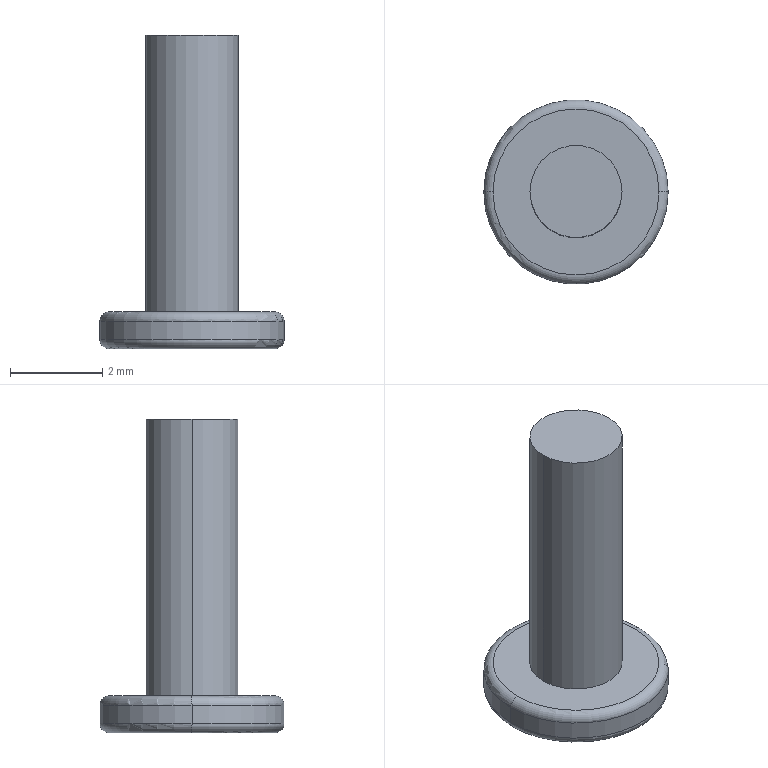Part | NX | features BREP 1 | 1 solid | 24 faces | box 4 x 4 x 6.8 mm | volume 27.69 mm3 | plane 10 | cone 6 | torus 4 | cylinder 4 | commonest cylinder face diameters 2 x2 4 x2
STEP:
#1=CARTESIAN_POINT('',(-2.,0.,0.6));
#2=VERTEX_POINT('',#1);
#3=CARTESIAN_POINT('',(2.,0.,0.6));
#4=VERTEX_POINT('',#3);
#5=CARTESIAN_POINT('',(0.,0.,0.6));
#6=DIRECTION('',(0.,0.,-1.));
#7=DIRECTION('',(1.,0.,0.));
#8=AXIS2_PLACEMENT_3D('',#5,#6,#7);
#9=CIRCLE('',#8,2.);
#10=EDGE_CURVE('',#2,#4,#9,.T.);
#11=ORIENTED_EDGE('',*,*,#10,.F.);
#12=CARTESIAN_POINT('',(-1.8,0.,0.8));
#13=VERTEX_POINT('',#12);
#14=CARTESIAN_POINT('',(-1.8,0.,0.6));
#15=DIRECTION('',(0.,1.,0.));
#16=DIRECTION('',(-1.,0.,0.));
#17=AXIS2_PLACEMENT_3D('',#14,#15,#16);
#18=CIRCLE('',#17,0.2);
#19=EDGE_CURVE('',#2,#13,#18,.T.);
#20=ORIENTED_EDGE('',*,*,#19,.T.);
#21=CARTESIAN_POINT('',(1.8,0.,0.8));
#22=VERTEX_POINT('',#21);
#23=CARTESIAN_POINT('',(0.,0.,0.8));
#24=DIRECTION('',(0.,0.,1.));
#25=DIRECTION('',(1.,0.,0.));
#26=AXIS2_PLACEMENT_3D('',#23,#24,#25);
#27=CIRCLE('',#26,1.8);
#28=EDGE_CURVE('',#22,#13,#27,.T.);
#29=ORIENTED_EDGE('',*,*,#28,.F.);
#30=CARTESIAN_POINT('',(1.8,0.,0.6));
#31=DIRECTION('',(0.,-1.,0.));
#32=DIRECTION('',(0.,0.,-1.));
#33=AXIS2_PLACEMENT_3D('',#30,#31,#32);
#34=CIRCLE('',#33,0.2);
#35=EDGE_CURVE('',#4,#22,#34,.T.);
#36=ORIENTED_EDGE('',*,*,#35,.F.);
#37=EDGE_LOOP('',(#11,#20,#29,#36));
#38=FACE_BOUND('',#37,.T.);
#39=CARTESIAN_POINT('',(0.,0.,0.6));
#40=DIRECTION('',(0.,0.,1.));
#41=DIRECTION('',(-1.,0.,0.));
#42=AXIS2_PLACEMENT_3D('',#39,#40,#41);
#43=TOROIDAL_SURFACE('',#42,1.8,0.2);
#44=ADVANCED_FACE('',(#38),#43,.T.);
#45=CARTESIAN_POINT('',(-1.8,0.,0.));
#46=VERTEX_POINT('',#45);
#47=CARTESIAN_POINT('',(1.8,0.,0.));
#48=VERTEX_POINT('',#47);
#49=CARTESIAN_POINT('',(0.,0.,0.));
#50=DIRECTION('',(0.,0.,-1.));
#51=DIRECTION('',(1.,0.,0.));
#52=AXIS2_PLACEMENT_3D('',#49,#50,#51);
#53=CIRCLE('',#52,1.8);
#54=EDGE_CURVE('',#46,#48,#53,.T.);
#55=ORIENTED_EDGE('',*,*,#54,.F.);
#56=CARTESIAN_POINT('',(-2.,0.,0.2));
#57=VERTEX_POINT('',#56);
#58=CARTESIAN_POINT('',(-1.8,0.,0.2));
#59=DIRECTION('',(0.,1.,0.));
#60=DIRECTION('',(-1.,0.,0.));
#61=AXIS2_PLACEMENT_3D('',#58,#59,#60);
#62=CIRCLE('',#61,0.2);
#63=EDGE_CURVE('',#46,#57,#62,.T.);
#64=ORIENTED_EDGE('',*,*,#63,.T.);
#65=CARTESIAN_POINT('',(2.,0.,0.2));
#66=VERTEX_POINT('',#65);
#67=CARTESIAN_POINT('',(0.,0.,0.2));
#68=DIRECTION('',(0.,0.,1.));
#69=DIRECTION('',(1.,0.,0.));
#70=AXIS2_PLACEMENT_3D('',#67,#68,#69);
#71=CIRCLE('',#70,2.);
#72=EDGE_CURVE('',#66,#57,#71,.T.);
#73=ORIENTED_EDGE('',*,*,#72,.F.);
#74=CARTESIAN_POINT('',(1.8,0.,0.2));
#75=DIRECTION('',(0.,-1.,0.));
#76=DIRECTION('',(0.,0.,-1.));
#77=AXIS2_PLACEMENT_3D('',#74,#75,#76);
#78=CIRCLE('',#77,0.2);
#79=EDGE_CURVE('',#48,#66,#78,.T.);
#80=ORIENTED_EDGE('',*,*,#79,.F.);
#81=EDGE_LOOP('',(#55,#64,#73,#80));
#82=FACE_BOUND('',#81,.T.);
#83=CARTESIAN_POINT('',(0.,0.,0.2));
#84=DIRECTION('',(0.,0.,1.));
#85=DIRECTION('',(-1.,0.,0.));
#86=AXIS2_PLACEMENT_3D('',#83,#84,#85);
#87=TOROIDAL_SURFACE('',#86,1.8,0.2);
#88=ADVANCED_FACE('',(#82),#87,.T.);
#89=CARTESIAN_POINT('',(1.,0.,6.8));
#90=VERTEX_POINT('',#89);
#91=CARTESIAN_POINT('',(-1.,0.,6.8));
#92=VERTEX_POINT('',#91);
#93=CARTESIAN_POINT('',(0.,0.,6.8));
#94=DIRECTION('',(0.,0.,1.));
#95=DIRECTION('',(1.,0.,0.));
#96=AXIS2_PLACEMENT_3D('',#93,#94,#95);
#97=CIRCLE('',#96,1.);
#98=EDGE_CURVE('',#90,#92,#97,.T.);
#99=ORIENTED_EDGE('',*,*,#98,.F.);
#100=CARTESIAN_POINT('',(1.,0.,0.8));
#101=VERTEX_POINT('',#100);
#102=CARTESIAN_POINT('',(1.,0.,6.8));
#103=DIRECTION('',(0.,0.,-1.));
#104=VECTOR('',#103,1000.);
#105=LINE('',#102,#104);
#106=EDGE_CURVE('',#101,#90,#105,.F.);
#107=ORIENTED_EDGE('',*,*,#106,.F.);
#108=CARTESIAN_POINT('',(-1.,0.,0.8));
#109=VERTEX_POINT('',#108);
#110=CARTESIAN_POINT('',(0.,0.,0.8));
#111=DIRECTION('',(0.,0.,1.));
#112=DIRECTION('',(1.,0.,0.));
#113=AXIS2_PLACEMENT_3D('',#110,#111,#112);
#114=CIRCLE('',#113,1.);
#115=EDGE_CURVE('',#101,#109,#114,.T.);
#116=ORIENTED_EDGE('',*,*,#115,.T.);
#117=CARTESIAN_POINT('',(-1.,0.,6.8));
#118=DIRECTION('',(0.,0.,-1.));
#119=VECTOR('',#118,1000.);
#120=LINE('',#117,#119);
#121=EDGE_CURVE('',#109,#92,#120,.F.);
#122=ORIENTED_EDGE('',*,*,#121,.T.);
#123=EDGE_LOOP('',(#99,#107,#116,#122));
#124=FACE_BOUND('',#123,.T.);
#125=CARTESIAN_POINT('',(0.,0.,6.8));
#126=DIRECTION('',(0.,0.,-1.));
#127=DIRECTION('',(1.,0.,0.));
#128=AXIS2_PLACEMENT_3D('',#125,#126,#127);
#129=CYLINDRICAL_SURFACE('',#128,1.);
#130=ADVANCED_FACE('',(#124),#129,.T.);
#131=ORIENTED_EDGE('',*,*,#10,.T.);
#132=CARTESIAN_POINT('',(2.,0.,0.8));
#133=DIRECTION('',(0.,0.,-1.));
#134=VECTOR('',#133,1000.);
#135=LINE('',#132,#134);
#136=EDGE_CURVE('',#66,#4,#135,.F.);
#137=ORIENTED_EDGE('',*,*,#136,.F.);
#138=ORIENTED_EDGE('',*,*,#72,.T.);
#139=CARTESIAN_POINT('',(-2.,0.,0.8));
#140=DIRECTION('',(0.,0.,-1.));
#141=VECTOR('',#140,1000.);
#142=LINE('',#139,#141);
#143=EDGE_CURVE('',#57,#2,#142,.F.);
#144=ORIENTED_EDGE('',*,*,#143,.T.);
#145=EDGE_LOOP('',(#131,#137,#138,#144));
#146=FACE_BOUND('',#145,.T.);
#147=CARTESIAN_POINT('',(0.,0.,0.8));
#148=DIRECTION('',(0.,0.,-1.));
#149=DIRECTION('',(1.,0.,0.));
#150=AXIS2_PLACEMENT_3D('',#147,#148,#149);
#151=CYLINDRICAL_SURFACE('',#150,2.);
#152=ADVANCED_FACE('',(#146),#151,.T.);
#153=ORIENTED_EDGE('',*,*,#136,.T.);
#154=CARTESIAN_POINT('',(0.,0.,0.6));
#155=DIRECTION('',(0.,0.,-1.));
#156=DIRECTION('',(1.,0.,0.));
#157=AXIS2_PLACEMENT_3D('',#154,#155,#156);
#158=CIRCLE('',#157,2.);
#159=EDGE_CURVE('',#4,#2,#158,.T.);
#160=ORIENTED_EDGE('',*,*,#159,.T.);
#161=ORIENTED_EDGE('',*,*,#143,.F.);
#162=CARTESIAN_POINT('',(0.,0.,0.2));
#163=DIRECTION('',(0.,0.,1.));
#164=DIRECTION('',(1.,0.,0.));
#165=AXIS2_PLACEMENT_3D('',#162,#163,#164);
#166=CIRCLE('',#165,2.);
#167=EDGE_CURVE('',#57,#66,#166,.T.);
#168=ORIENTED_EDGE('',*,*,#167,.T.);
#169=EDGE_LOOP('',(#153,#160,#161,#168));
#170=FACE_BOUND('',#169,.T.);
#171=CARTESIAN_POINT('',(0.,0.,0.8));
#172=DIRECTION('',(0.,0.,-1.));
#173=DIRECTION('',(1.,0.,0.));
#174=AXIS2_PLACEMENT_3D('',#171,#172,#173);
#175=CYLINDRICAL_SURFACE('',#174,2.);
#176=ADVANCED_FACE('',(#170),#175,.T.);
#177=ORIENTED_EDGE('',*,*,#28,.T.);
#178=CARTESIAN_POINT('',(0.,0.,0.8));
#179=DIRECTION('',(0.,0.,1.));
#180=DIRECTION('',(1.,0.,0.));
#181=AXIS2_PLACEMENT_3D('',#178,#179,#180);
#182=CIRCLE('',#181,1.8);
#183=EDGE_CURVE('',#13,#22,#182,.T.);
#184=ORIENTED_EDGE('',*,*,#183,.T.);
#185=EDGE_LOOP('',(#177,#184));
#186=FACE_BOUND('',#185,.T.);
#187=CARTESIAN_POINT('',(0.,0.,0.8));
#188=DIRECTION('',(0.,0.,1.));
#189=DIRECTION('',(1.,0.,0.));
#190=AXIS2_PLACEMENT_3D('',#187,#188,#189);
#191=CIRCLE('',#190,1.);
#192=EDGE_CURVE('',#109,#101,#191,.T.);
#193=ORIENTED_EDGE('',*,*,#192,.F.);
#194=ORIENTED_EDGE('',*,*,#115,.F.);
#195=EDGE_LOOP('',(#193,#194));
#196=FACE_BOUND('',#195,.T.);
#197=CARTESIAN_POINT('',(0.,0.,0.8));
#198=DIRECTION('',(0.,0.,1.));
#199=DIRECTION('',(-1.,0.,0.));
#200=AXIS2_PLACEMENT_3D('',#197,#198,#199);
#201=PLANE('',#200);
#202=ADVANCED_FACE('',(#186,#196),#201,.T.);
#203=CARTESIAN_POINT('',(0.,0.,0.));
#204=DIRECTION('',(0.,0.,-1.));
#205=DIRECTION('',(1.,0.,0.));
#206=AXIS2_PLACEMENT_3D('',#203,#204,#205);
#207=CIRCLE('',#206,1.8);
#208=EDGE_CURVE('',#48,#46,#207,.T.);
#209=ORIENTED_EDGE('',*,*,#208,.T.);
#210=ORIENTED_EDGE('',*,*,#54,.T.);
#211=EDGE_LOOP('',(#209,#210));
#212=FACE_BOUND('',#211,.T.);
#213=CARTESIAN_POINT('',(0.866,0.,0.));
#214=VERTEX_POINT('',#213);
#215=CARTESIAN_POINT('',(0.433,-0.75,0.));
#216=VERTEX_POINT('',#215);
#217=CARTESIAN_POINT('',(0.,0.,0.));
#218=DIRECTION('',(0.,0.,-1.));
#219=DIRECTION('',(-1.,0.,0.));
#220=AXIS2_PLACEMENT_3D('',#217,#218,#219);
#221=CIRCLE('',#220,0.866);
#222=EDGE_CURVE('',#214,#216,#221,.T.);
#223=ORIENTED_EDGE('',*,*,#222,.F.);
#224=CARTESIAN_POINT('',(0.433,0.75,0.));
#225=VERTEX_POINT('',#224);
#226=CARTESIAN_POINT('',(0.,0.,0.));
#227=DIRECTION('',(0.,0.,-1.));
#228=DIRECTION('',(-1.,0.,0.));
#229=AXIS2_PLACEMENT_3D('',#226,#227,#228);
#230=CIRCLE('',#229,0.866);
#231=EDGE_CURVE('',#225,#214,#230,.T.);
#232=ORIENTED_EDGE('',*,*,#231,.F.);
#233=CARTESIAN_POINT('',(-0.433,0.75,0.));
#234=VERTEX_POINT('',#233);
#235=CARTESIAN_POINT('',(0.,0.,0.));
#236=DIRECTION('',(0.,0.,-1.));
#237=DIRECTION('',(-1.,0.,0.));
#238=AXIS2_PLACEMENT_3D('',#235,#236,#237);
#239=CIRCLE('',#238,0.866);
#240=EDGE_CURVE('',#234,#225,#239,.T.);
#241=ORIENTED_EDGE('',*,*,#240,.F.);
#242=CARTESIAN_POINT('',(-0.866,0.,0.));
#243=VERTEX_POINT('',#242);
#244=CARTESIAN_POINT('',(0.,0.,0.));
#245=DIRECTION('',(0.,0.,-1.));
#246=DIRECTION('',(-1.,0.,0.));
#247=AXIS2_PLACEMENT_3D('',#244,#245,#246);
#248=CIRCLE('',#247,0.866);
#249=EDGE_CURVE('',#243,#234,#248,.T.);
#250=ORIENTED_EDGE('',*,*,#249,.F.);
#251=CARTESIAN_POINT('',(-0.433,-0.75,0.));
#252=VERTEX_POINT('',#251);
#253=CARTESIAN_POINT('',(0.,0.,0.));
#254=DIRECTION('',(0.,0.,-1.));
#255=DIRECTION('',(-1.,0.,0.));
#256=AXIS2_PLACEMENT_3D('',#253,#254,#255);
#257=CIRCLE('',#256,0.866);
#258=EDGE_CURVE('',#252,#243,#257,.T.);
#259=ORIENTED_EDGE('',*,*,#258,.F.);
#260=CARTESIAN_POINT('',(0.,0.,0.));
#261=DIRECTION('',(0.,0.,-1.));
#262=DIRECTION('',(-1.,0.,0.));
#263=AXIS2_PLACEMENT_3D('',#260,#261,#262);
#264=CIRCLE('',#263,0.866);
#265=EDGE_CURVE('',#216,#252,#264,.T.);
#266=ORIENTED_EDGE('',*,*,#265,.F.);
#267=EDGE_LOOP('',(#223,#232,#241,#250,#259,#266));
#268=FACE_BOUND('',#267,.T.);
#269=CARTESIAN_POINT('',(0.,0.,0.));
#270=DIRECTION('',(0.,0.,1.));
#271=DIRECTION('',(-1.,0.,0.));
#272=AXIS2_PLACEMENT_3D('',#269,#270,#271);
#273=PLANE('',#272);
#274=ADVANCED_FACE('',(#212,#268),#273,.F.);
#275=ORIENTED_EDGE('',*,*,#106,.T.);
#276=CARTESIAN_POINT('',(0.,0.,6.8));
#277=DIRECTION('',(0.,0.,1.));
#278=DIRECTION('',(1.,0.,0.));
#279=AXIS2_PLACEMENT_3D('',#276,#277,#278);
#280=CIRCLE('',#279,1.);
#281=EDGE_CURVE('',#92,#90,#280,.T.);
#282=ORIENTED_EDGE('',*,*,#281,.F.);
#283=ORIENTED_EDGE('',*,*,#121,.F.);
#284=ORIENTED_EDGE('',*,*,#192,.T.);
#285=EDGE_LOOP('',(#275,#282,#283,#284));
#286=FACE_BOUND('',#285,.T.);
#287=CARTESIAN_POINT('',(0.,0.,6.8));
#288=DIRECTION('',(0.,0.,-1.));
#289=DIRECTION('',(1.,0.,0.));
#290=AXIS2_PLACEMENT_3D('',#287,#288,#289);
#291=CYLINDRICAL_SURFACE('',#290,1.);
#292=ADVANCED_FACE('',(#286),#291,.T.);
#293=ORIENTED_EDGE('',*,*,#281,.T.);
#294=ORIENTED_EDGE('',*,*,#98,.T.);
#295=EDGE_LOOP('',(#293,#294));
#296=FACE_BOUND('',#295,.T.);
#297=CARTESIAN_POINT('',(0.,0.,6.8));
#298=DIRECTION('',(0.,0.,1.));
#299=DIRECTION('',(-1.,0.,0.));
#300=AXIS2_PLACEMENT_3D('',#297,#298,#299);
#301=PLANE('',#300);
#302=ADVANCED_FACE('',(#296),#301,.T.);
#303=ORIENTED_EDGE('',*,*,#249,.T.);
#304=CARTESIAN_POINT('',(-0.866,0.,0.));
#305=CARTESIAN_POINT('',(-0.7307,0.2344,0.1353));
#306=CARTESIAN_POINT('',(-0.5691,0.5142,0.1361));
#307=CARTESIAN_POINT('',(-0.433,0.75,0.));
#308=B_SPLINE_CURVE_WITH_KNOTS('',3,(#304,#305,#306,#307),.UNSPECIFIED.,.F.,.F.,(4,4),(0.,0.0008946),.UNSPECIFIED.);
#309=EDGE_CURVE('',#243,#234,#308,.T.);
#310=ORIENTED_EDGE('',*,*,#309,.F.);
#311=EDGE_LOOP('',(#303,#310));
#312=FACE_BOUND('',#311,.T.);
#313=CARTESIAN_POINT('',(0.,0.,0.));
#314=DIRECTION('',(0.,0.,-1.));
#315=DIRECTION('',(1.,0.,0.));
#316=AXIS2_PLACEMENT_3D('',#313,#314,#315);
#317=CONICAL_SURFACE('',#316,0.866,0.7854);
#318=ADVANCED_FACE('',(#312),#317,.F.);
#319=ORIENTED_EDGE('',*,*,#240,.T.);
#320=CARTESIAN_POINT('',(-0.433,0.75,0.));
#321=CARTESIAN_POINT('',(-0.1624,0.75,0.1353));
#322=CARTESIAN_POINT('',(0.1608,0.75,0.1361));
#323=CARTESIAN_POINT('',(0.433,0.75,0.));
#324=B_SPLINE_CURVE_WITH_KNOTS('',3,(#320,#321,#322,#323),.UNSPECIFIED.,.F.,.F.,(4,4),(0.,0.0008946),.UNSPECIFIED.);
#325=EDGE_CURVE('',#234,#225,#324,.T.);
#326=ORIENTED_EDGE('',*,*,#325,.F.);
#327=EDGE_LOOP('',(#319,#326));
#328=FACE_BOUND('',#327,.T.);
#329=CARTESIAN_POINT('',(0.,0.,0.));
#330=DIRECTION('',(0.,0.,-1.));
#331=DIRECTION('',(1.,0.,0.));
#332=AXIS2_PLACEMENT_3D('',#329,#330,#331);
#333=CONICAL_SURFACE('',#332,0.866,0.7854);
#334=ADVANCED_FACE('',(#328),#333,.F.);
#335=ORIENTED_EDGE('',*,*,#231,.T.);
#336=CARTESIAN_POINT('',(0.433,0.75,0.));
#337=CARTESIAN_POINT('',(0.5683,0.5156,0.1353));
#338=CARTESIAN_POINT('',(0.7299,0.2358,0.1361));
#339=CARTESIAN_POINT('',(0.866,0.,0.));
#340=B_SPLINE_CURVE_WITH_KNOTS('',3,(#336,#337,#338,#339),.UNSPECIFIED.,.F.,.F.,(4,4),(0.,0.0008946),.UNSPECIFIED.);
#341=EDGE_CURVE('',#225,#214,#340,.T.);
#342=ORIENTED_EDGE('',*,*,#341,.F.);
#343=EDGE_LOOP('',(#335,#342));
#344=FACE_BOUND('',#343,.T.);
#345=CARTESIAN_POINT('',(0.,0.,0.));
#346=DIRECTION('',(0.,0.,-1.));
#347=DIRECTION('',(1.,0.,0.));
#348=AXIS2_PLACEMENT_3D('',#345,#346,#347);
#349=CONICAL_SURFACE('',#348,0.866,0.7854);
#350=ADVANCED_FACE('',(#344),#349,.F.);
#351=ORIENTED_EDGE('',*,*,#222,.T.);
#352=CARTESIAN_POINT('',(0.866,0.,0.));
#353=CARTESIAN_POINT('',(0.7307,-0.2344,0.1353));
#354=CARTESIAN_POINT('',(0.5691,-0.5142,0.1361));
#355=CARTESIAN_POINT('',(0.433,-0.75,0.));
#356=B_SPLINE_CURVE_WITH_KNOTS('',3,(#352,#353,#354,#355),.UNSPECIFIED.,.F.,.F.,(4,4),(0.,0.0008946),.UNSPECIFIED.);
#357=EDGE_CURVE('',#214,#216,#356,.T.);
#358=ORIENTED_EDGE('',*,*,#357,.F.);
#359=EDGE_LOOP('',(#351,#358));
#360=FACE_BOUND('',#359,.T.);
#361=CARTESIAN_POINT('',(0.,0.,0.));
#362=DIRECTION('',(0.,0.,-1.));
#363=DIRECTION('',(1.,0.,0.));
#364=AXIS2_PLACEMENT_3D('',#361,#362,#363);
#365=CONICAL_SURFACE('',#364,0.866,0.7854);
#366=ADVANCED_FACE('',(#360),#365,.F.);
#367=ORIENTED_EDGE('',*,*,#265,.T.);
#368=CARTESIAN_POINT('',(0.433,-0.75,0.));
#369=CARTESIAN_POINT('',(0.1624,-0.75,0.1353));
#370=CARTESIAN_POINT('',(-0.1608,-0.75,0.1361));
#371=CARTESIAN_POINT('',(-0.433,-0.75,0.));
#372=B_SPLINE_CURVE_WITH_KNOTS('',3,(#368,#369,#370,#371),.UNSPECIFIED.,.F.,.F.,(4,4),(0.,0.0008946),.UNSPECIFIED.);
#373=EDGE_CURVE('',#216,#252,#372,.T.);
#374=ORIENTED_EDGE('',*,*,#373,.F.);
#375=EDGE_LOOP('',(#367,#374));
#376=FACE_BOUND('',#375,.T.);
#377=CARTESIAN_POINT('',(0.,0.,0.));
#378=DIRECTION('',(0.,0.,-1.));
#379=DIRECTION('',(1.,0.,0.));
#380=AXIS2_PLACEMENT_3D('',#377,#378,#379);
#381=CONICAL_SURFACE('',#380,0.866,0.7854);
#382=ADVANCED_FACE('',(#376),#381,.F.);
#383=ORIENTED_EDGE('',*,*,#258,.T.);
#384=CARTESIAN_POINT('',(-0.433,-0.75,0.));
#385=CARTESIAN_POINT('',(-0.5683,-0.5156,0.1353));
#386=CARTESIAN_POINT('',(-0.7299,-0.2358,0.1361));
#387=CARTESIAN_POINT('',(-0.866,0.,0.));
#388=B_SPLINE_CURVE_WITH_KNOTS('',3,(#384,#385,#386,#387),.UNSPECIFIED.,.F.,.F.,(4,4),(0.,0.0008946),.UNSPECIFIED.);
#389=EDGE_CURVE('',#252,#243,#388,.T.);
#390=ORIENTED_EDGE('',*,*,#389,.F.);
#391=EDGE_LOOP('',(#383,#390));
#392=FACE_BOUND('',#391,.T.);
#393=CARTESIAN_POINT('',(0.,0.,0.));
#394=DIRECTION('',(0.,0.,-1.));
#395=DIRECTION('',(1.,0.,0.));
#396=AXIS2_PLACEMENT_3D('',#393,#394,#395);
#397=CONICAL_SURFACE('',#396,0.866,0.7854);
#398=ADVANCED_FACE('',(#392),#397,.F.);
#399=CARTESIAN_POINT('',(-0.433,-0.75,0.5));
#400=VERTEX_POINT('',#399);
#401=CARTESIAN_POINT('',(-0.866,0.,0.5));
#402=VERTEX_POINT('',#401);
#403=CARTESIAN_POINT('',(-0.433,-0.75,0.5));
#404=DIRECTION('',(-0.5,0.866,0.));
#405=VECTOR('',#404,1000.);
#406=LINE('',#403,#405);
#407=EDGE_CURVE('',#400,#402,#406,.T.);
#408=ORIENTED_EDGE('',*,*,#407,.T.);
#409=CARTESIAN_POINT('',(-0.433,0.75,0.5));
#410=VERTEX_POINT('',#409);
#411=CARTESIAN_POINT('',(-0.866,0.,0.5));
#412=DIRECTION('',(0.5,0.866,0.));
#413=VECTOR('',#412,1000.);
#414=LINE('',#411,#413);
#415=EDGE_CURVE('',#402,#410,#414,.T.);
#416=ORIENTED_EDGE('',*,*,#415,.T.);
#417=CARTESIAN_POINT('',(0.433,0.75,0.5));
#418=VERTEX_POINT('',#417);
#419=CARTESIAN_POINT('',(-0.433,0.75,0.5));
#420=DIRECTION('',(1.,0.,0.));
#421=VECTOR('',#420,1000.);
#422=LINE('',#419,#421);
#423=EDGE_CURVE('',#410,#418,#422,.T.);
#424=ORIENTED_EDGE('',*,*,#423,.T.);
#425=CARTESIAN_POINT('',(0.866,0.,0.5));
#426=VERTEX_POINT('',#425);
#427=CARTESIAN_POINT('',(0.433,0.75,0.5));
#428=DIRECTION('',(0.5,-0.866,0.));
#429=VECTOR('',#428,1000.);
#430=LINE('',#427,#429);
#431=EDGE_CURVE('',#418,#426,#430,.T.);
#432=ORIENTED_EDGE('',*,*,#431,.T.);
#433=CARTESIAN_POINT('',(0.433,-0.75,0.5));
#434=VERTEX_POINT('',#433);
#435=CARTESIAN_POINT('',(0.866,0.,0.5));
#436=DIRECTION('',(-0.5,-0.866,0.));
#437=VECTOR('',#436,1000.);
#438=LINE('',#435,#437);
#439=EDGE_CURVE('',#426,#434,#438,.T.);
#440=ORIENTED_EDGE('',*,*,#439,.T.);
#441=CARTESIAN_POINT('',(0.433,-0.75,0.5));
#442=DIRECTION('',(-1.,0.,0.));
#443=VECTOR('',#442,1000.);
#444=LINE('',#441,#443);
#445=EDGE_CURVE('',#434,#400,#444,.T.);
#446=ORIENTED_EDGE('',*,*,#445,.T.);
#447=EDGE_LOOP('',(#408,#416,#424,#432,#440,#446));
#448=FACE_BOUND('',#447,.T.);
#449=CARTESIAN_POINT('',(0.,0.,0.5));
#450=DIRECTION('',(0.,0.,-1.));
#451=DIRECTION('',(0.,1.,0.));
#452=AXIS2_PLACEMENT_3D('',#449,#450,#451);
#453=PLANE('',#452);
#454=ADVANCED_FACE('',(#448),#453,.T.);
#455=CARTESIAN_POINT('',(-0.866,0.,0.5));
#456=DIRECTION('',(0.,0.,-1.));
#457=VECTOR('',#456,1000.);
#458=LINE('',#455,#457);
#459=EDGE_CURVE('',#402,#243,#458,.T.);
#460=ORIENTED_EDGE('',*,*,#459,.T.);
#461=ORIENTED_EDGE('',*,*,#309,.T.);
#462=CARTESIAN_POINT('',(-0.433,0.75,0.5));
#463=DIRECTION('',(0.,0.,-1.));
#464=VECTOR('',#463,1000.);
#465=LINE('',#462,#464);
#466=EDGE_CURVE('',#410,#234,#465,.T.);
#467=ORIENTED_EDGE('',*,*,#466,.F.);
#468=ORIENTED_EDGE('',*,*,#415,.F.);
#469=EDGE_LOOP('',(#460,#461,#467,#468));
#470=FACE_BOUND('',#469,.T.);
#471=CARTESIAN_POINT('',(-0.866,0.,0.5));
#472=DIRECTION('',(-0.866,0.5,0.));
#473=DIRECTION('',(0.,0.,-1.));
#474=AXIS2_PLACEMENT_3D('',#471,#472,#473);
#475=PLANE('',#474);
#476=ADVANCED_FACE('',(#470),#475,.F.);
#477=ORIENTED_EDGE('',*,*,#466,.T.);
#478=ORIENTED_EDGE('',*,*,#325,.T.);
#479=CARTESIAN_POINT('',(0.433,0.75,0.5));
#480=DIRECTION('',(0.,0.,-1.));
#481=VECTOR('',#480,1000.);
#482=LINE('',#479,#481);
#483=EDGE_CURVE('',#418,#225,#482,.T.);
#484=ORIENTED_EDGE('',*,*,#483,.F.);
#485=ORIENTED_EDGE('',*,*,#423,.F.);
#486=EDGE_LOOP('',(#477,#478,#484,#485));
#487=FACE_BOUND('',#486,.T.);
#488=CARTESIAN_POINT('',(-0.433,0.75,0.5));
#489=DIRECTION('',(0.,1.,0.));
#490=DIRECTION('',(-1.,0.,0.));
#491=AXIS2_PLACEMENT_3D('',#488,#489,#490);
#492=PLANE('',#491);
#493=ADVANCED_FACE('',(#487),#492,.F.);
#494=ORIENTED_EDGE('',*,*,#483,.T.);
#495=ORIENTED_EDGE('',*,*,#341,.T.);
#496=CARTESIAN_POINT('',(0.866,0.,0.5));
#497=DIRECTION('',(0.,0.,-1.));
#498=VECTOR('',#497,1000.);
#499=LINE('',#496,#498);
#500=EDGE_CURVE('',#426,#214,#499,.T.);
#501=ORIENTED_EDGE('',*,*,#500,.F.);
#502=ORIENTED_EDGE('',*,*,#431,.F.);
#503=EDGE_LOOP('',(#494,#495,#501,#502));
#504=FACE_BOUND('',#503,.T.);
#505=CARTESIAN_POINT('',(0.433,0.75,0.5));
#506=DIRECTION('',(0.866,0.5,0.));
#507=DIRECTION('',(0.,0.,1.));
#508=AXIS2_PLACEMENT_3D('',#505,#506,#507);
#509=PLANE('',#508);
#510=ADVANCED_FACE('',(#504),#509,.F.);
#511=ORIENTED_EDGE('',*,*,#500,.T.);
#512=ORIENTED_EDGE('',*,*,#357,.T.);
#513=CARTESIAN_POINT('',(0.433,-0.75,0.5));
#514=DIRECTION('',(0.,0.,-1.));
#515=VECTOR('',#514,1000.);
#516=LINE('',#513,#515);
#517=EDGE_CURVE('',#434,#216,#516,.T.);
#518=ORIENTED_EDGE('',*,*,#517,.F.);
#519=ORIENTED_EDGE('',*,*,#439,.F.);
#520=EDGE_LOOP('',(#511,#512,#518,#519));
#521=FACE_BOUND('',#520,.T.);
#522=CARTESIAN_POINT('',(0.866,0.,0.5));
#523=DIRECTION('',(0.866,-0.5,0.));
#524=DIRECTION('',(0.,0.,1.));
#525=AXIS2_PLACEMENT_3D('',#522,#523,#524);
#526=PLANE('',#525);
#527=ADVANCED_FACE('',(#521),#526,.F.);
#528=ORIENTED_EDGE('',*,*,#517,.T.);
#529=ORIENTED_EDGE('',*,*,#373,.T.);
#530=CARTESIAN_POINT('',(-0.433,-0.75,0.5));
#531=DIRECTION('',(0.,0.,-1.));
#532=VECTOR('',#531,1000.);
#533=LINE('',#530,#532);
#534=EDGE_CURVE('',#400,#252,#533,.T.);
#535=ORIENTED_EDGE('',*,*,#534,.F.);
#536=ORIENTED_EDGE('',*,*,#445,.F.);
#537=EDGE_LOOP('',(#528,#529,#535,#536));
#538=FACE_BOUND('',#537,.T.);
#539=CARTESIAN_POINT('',(0.433,-0.75,0.5));
#540=DIRECTION('',(0.,-1.,0.));
#541=DIRECTION('',(0.,0.,1.));
#542=AXIS2_PLACEMENT_3D('',#539,#540,#541);
#543=PLANE('',#542);
#544=ADVANCED_FACE('',(#538),#543,.F.);
#545=ORIENTED_EDGE('',*,*,#534,.T.);
#546=ORIENTED_EDGE('',*,*,#389,.T.);
#547=ORIENTED_EDGE('',*,*,#459,.F.);
#548=ORIENTED_EDGE('',*,*,#407,.F.);
#549=EDGE_LOOP('',(#545,#546,#547,#548));
#550=FACE_BOUND('',#549,.T.);
#551=CARTESIAN_POINT('',(-0.433,-0.75,0.5));
#552=DIRECTION('',(-0.866,-0.5,0.));
#553=DIRECTION('',(0.5,-0.866,0.));
#554=AXIS2_PLACEMENT_3D('',#551,#552,#553);
#555=PLANE('',#554);
#556=ADVANCED_FACE('',(#550),#555,.F.);
#557=ORIENTED_EDGE('',*,*,#63,.F.);
#558=ORIENTED_EDGE('',*,*,#208,.F.);
#559=ORIENTED_EDGE('',*,*,#79,.T.);
#560=ORIENTED_EDGE('',*,*,#167,.F.);
#561=EDGE_LOOP('',(#557,#558,#559,#560));
#562=FACE_BOUND('',#561,.T.);
#563=CARTESIAN_POINT('',(0.,0.,0.2));
#564=DIRECTION('',(0.,0.,1.));
#565=DIRECTION('',(-1.,0.,0.));
#566=AXIS2_PLACEMENT_3D('',#563,#564,#565);
#567=TOROIDAL_SURFACE('',#566,1.8,0.2);
#568=ADVANCED_FACE('',(#562),#567,.T.);
#569=ORIENTED_EDGE('',*,*,#19,.F.);
#570=ORIENTED_EDGE('',*,*,#159,.F.);
#571=ORIENTED_EDGE('',*,*,#35,.T.);
#572=ORIENTED_EDGE('',*,*,#183,.F.);
#573=EDGE_LOOP('',(#569,#570,#571,#572));
#574=FACE_BOUND('',#573,.T.);
#575=CARTESIAN_POINT('',(0.,0.,0.6));
#576=DIRECTION('',(0.,0.,1.));
#577=DIRECTION('',(-1.,0.,0.));
#578=AXIS2_PLACEMENT_3D('',#575,#576,#577);
#579=TOROIDAL_SURFACE('',#578,1.8,0.2);
#580=ADVANCED_FACE('',(#574),#579,.T.);
#581=CLOSED_SHELL('',(#44,#88,#130,#152,#176,#202,#274,#292,#302,#318,#334,#350,#366,#382,#398,#454,#476,#493,#510,#527,#544,#556,#568,#580));
#582=MANIFOLD_SOLID_BREP('',#581);
#583=(LENGTH_UNIT()NAMED_UNIT(*)SI_UNIT(.MILLI.,.METRE.));
#584=UNCERTAINTY_MEASURE_WITH_UNIT(LENGTH_MEASURE(0.0508),#583,'','');
#585=(NAMED_UNIT(*)PLANE_ANGLE_UNIT()SI_UNIT($,.RADIAN.));
#586=(NAMED_UNIT(*)SI_UNIT($,.STERADIAN.)SOLID_ANGLE_UNIT());
#587=(GEOMETRIC_REPRESENTATION_CONTEXT(3)GLOBAL_UNCERTAINTY_ASSIGNED_CONTEXT((#584))GLOBAL_UNIT_ASSIGNED_CONTEXT((#583,#585,#586))REPRESENTATION_CONTEXT('',''));
#588=ADVANCED_BREP_SHAPE_REPRESENTATION('',(#582),#587);